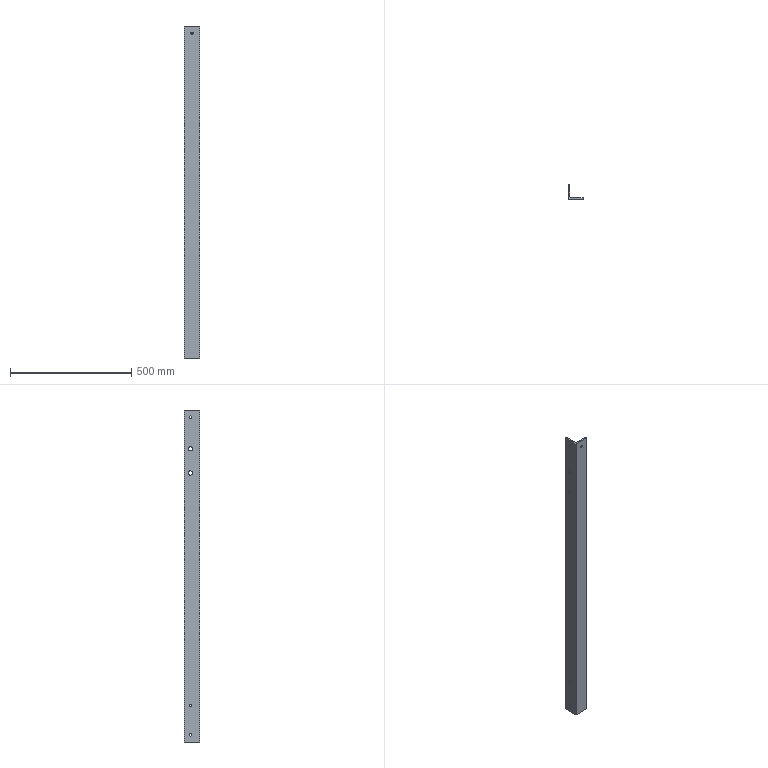Part | STEP file | 1 solid | 23 faces | box 63 x 63 x 1369 mm | volume 991989 mm3 | cylinder 15 | plane 8 | commonest cylinder face diameters 11 x6 17.5 x4 4.6 x2 9 x2 14 x1